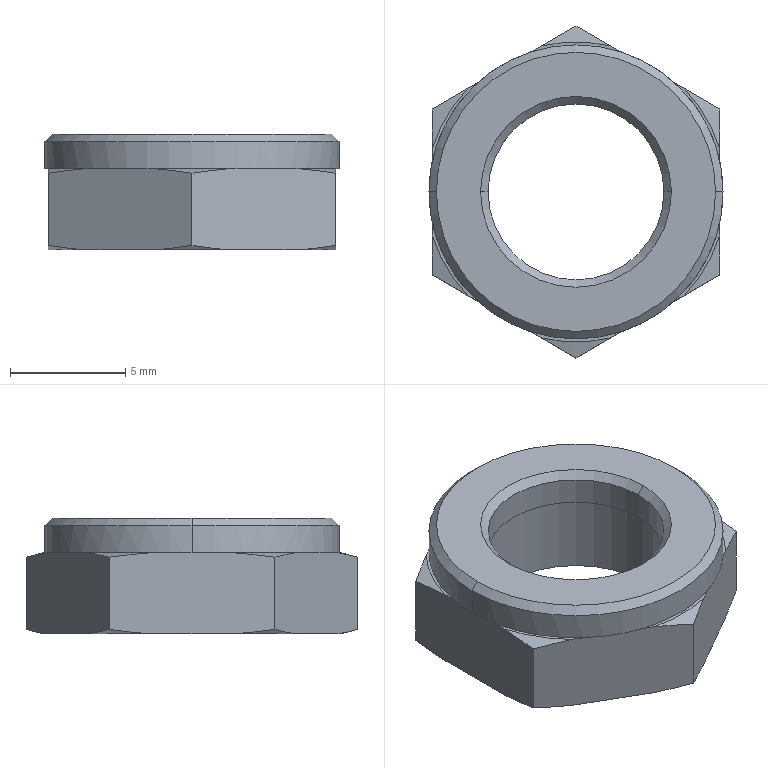Part | SolidWorks | features Cut 3, Boss 1, Chamfer 1, Extrusion 1 | 1 solid | 43 faces | box 12.74 x 14.38 x 5 mm | volume 412.934 mm3 | plane 21 | cone 16 | cylinder 6 | commonest cylinder face diameters 7.619 x2 8 x2 12.74 x2
STEP:
#1=CARTESIAN_POINT('',(-3.81,0.,4.675));
#2=VERTEX_POINT('',#1);
#3=CARTESIAN_POINT('',(3.81,0.,4.675));
#4=VERTEX_POINT('',#3);
#5=CARTESIAN_POINT('',(0.,0.,4.675));
#6=DIRECTION('',(0.,0.,1.));
#7=DIRECTION('',(1.,0.,0.));
#8=AXIS2_PLACEMENT_3D('',#5,#6,#7);
#9=CIRCLE('',#8,3.81);
#10=EDGE_CURVE('',#2,#4,#9,.T.);
#11=ORIENTED_EDGE('',*,*,#10,.F.);
#12=CARTESIAN_POINT('',(-4.135,0.,5.));
#13=VERTEX_POINT('',#12);
#14=CARTESIAN_POINT('',(-3.81,0.,4.675));
#15=DIRECTION('',(-0.7071,0.,0.7071));
#16=VECTOR('',#15,1000.);
#17=LINE('',#14,#16);
#18=EDGE_CURVE('',#2,#13,#17,.T.);
#19=ORIENTED_EDGE('',*,*,#18,.T.);
#20=CARTESIAN_POINT('',(4.135,0.,5.));
#21=VERTEX_POINT('',#20);
#22=CARTESIAN_POINT('',(0.,0.,5.));
#23=DIRECTION('',(0.,0.,-1.));
#24=DIRECTION('',(1.,0.,0.));
#25=AXIS2_PLACEMENT_3D('',#22,#23,#24);
#26=CIRCLE('',#25,4.135);
#27=EDGE_CURVE('',#21,#13,#26,.T.);
#28=ORIENTED_EDGE('',*,*,#27,.F.);
#29=CARTESIAN_POINT('',(3.81,0.,4.675));
#30=DIRECTION('',(0.7071,0.,0.7071));
#31=VECTOR('',#30,1000.);
#32=LINE('',#29,#31);
#33=EDGE_CURVE('',#4,#21,#32,.T.);
#34=ORIENTED_EDGE('',*,*,#33,.F.);
#35=EDGE_LOOP('',(#11,#19,#28,#34));
#36=FACE_OUTER_BOUND('',#35,.T.);
#37=CARTESIAN_POINT('',(0.,0.,4.675));
#38=DIRECTION('',(0.,0.,1.));
#39=DIRECTION('',(1.,0.,0.));
#40=AXIS2_PLACEMENT_3D('',#37,#38,#39);
#41=CONICAL_SURFACE('',#40,3.81,0.7854);
#42=ADVANCED_FACE('',(#36),#41,.F.);
#43=CARTESIAN_POINT('',(6.045,0.,5.));
#44=VERTEX_POINT('',#43);
#45=CARTESIAN_POINT('',(-6.045,0.,5.));
#46=VERTEX_POINT('',#45);
#47=CARTESIAN_POINT('',(0.,0.,5.));
#48=DIRECTION('',(0.,0.,1.));
#49=DIRECTION('',(1.,0.,0.));
#50=AXIS2_PLACEMENT_3D('',#47,#48,#49);
#51=CIRCLE('',#50,6.045);
#52=EDGE_CURVE('',#44,#46,#51,.T.);
#53=ORIENTED_EDGE('',*,*,#52,.F.);
#54=CARTESIAN_POINT('',(6.37,0.,4.675));
#55=VERTEX_POINT('',#54);
#56=CARTESIAN_POINT('',(6.045,0.,5.));
#57=DIRECTION('',(0.7071,0.,-0.7071));
#58=VECTOR('',#57,1000.);
#59=LINE('',#56,#58);
#60=EDGE_CURVE('',#44,#55,#59,.T.);
#61=ORIENTED_EDGE('',*,*,#60,.T.);
#62=CARTESIAN_POINT('',(-6.37,0.,4.675));
#63=VERTEX_POINT('',#62);
#64=CARTESIAN_POINT('',(0.,0.,4.675));
#65=DIRECTION('',(0.,0.,-1.));
#66=DIRECTION('',(1.,0.,0.));
#67=AXIS2_PLACEMENT_3D('',#64,#65,#66);
#68=CIRCLE('',#67,6.37);
#69=EDGE_CURVE('',#63,#55,#68,.T.);
#70=ORIENTED_EDGE('',*,*,#69,.F.);
#71=CARTESIAN_POINT('',(-6.045,0.,5.));
#72=DIRECTION('',(-0.7071,0.,-0.7071));
#73=VECTOR('',#72,1000.);
#74=LINE('',#71,#73);
#75=EDGE_CURVE('',#46,#63,#74,.T.);
#76=ORIENTED_EDGE('',*,*,#75,.F.);
#77=EDGE_LOOP('',(#53,#61,#70,#76));
#78=FACE_OUTER_BOUND('',#77,.T.);
#79=CARTESIAN_POINT('',(0.,0.,5.));
#80=DIRECTION('',(0.,0.,-1.));
#81=DIRECTION('',(-1.,0.,0.));
#82=AXIS2_PLACEMENT_3D('',#79,#80,#81);
#83=CONICAL_SURFACE('',#82,6.045,0.7854);
#84=ADVANCED_FACE('',(#78),#83,.T.);
#85=CARTESIAN_POINT('',(-3.81,0.,3.5));
#86=VERTEX_POINT('',#85);
#87=CARTESIAN_POINT('',(3.81,0.,3.5));
#88=VERTEX_POINT('',#87);
#89=CARTESIAN_POINT('',(0.,0.,3.5));
#90=DIRECTION('',(0.,0.,1.));
#91=DIRECTION('',(1.,0.,0.));
#92=AXIS2_PLACEMENT_3D('',#89,#90,#91);
#93=CIRCLE('',#92,3.81);
#94=EDGE_CURVE('',#86,#88,#93,.T.);
#95=ORIENTED_EDGE('',*,*,#94,.F.);
#96=CARTESIAN_POINT('',(-3.81,0.,0.));
#97=DIRECTION('',(0.,0.,1.));
#98=VECTOR('',#97,1000.);
#99=LINE('',#96,#98);
#100=EDGE_CURVE('',#86,#2,#99,.T.);
#101=ORIENTED_EDGE('',*,*,#100,.T.);
#102=ORIENTED_EDGE('',*,*,#10,.T.);
#103=CARTESIAN_POINT('',(3.81,0.,0.));
#104=DIRECTION('',(0.,0.,1.));
#105=VECTOR('',#104,1000.);
#106=LINE('',#103,#105);
#107=EDGE_CURVE('',#88,#4,#106,.T.);
#108=ORIENTED_EDGE('',*,*,#107,.F.);
#109=EDGE_LOOP('',(#95,#101,#102,#108));
#110=FACE_OUTER_BOUND('',#109,.T.);
#111=CARTESIAN_POINT('',(0.,0.,0.));
#112=DIRECTION('',(0.,0.,1.));
#113=DIRECTION('',(1.,0.,0.));
#114=AXIS2_PLACEMENT_3D('',#111,#112,#113);
#115=CYLINDRICAL_SURFACE('',#114,3.81);
#116=ADVANCED_FACE('',(#110),#115,.F.);
#117=ORIENTED_EDGE('',*,*,#69,.T.);
#118=CARTESIAN_POINT('',(6.37,0.,3.5));
#119=VERTEX_POINT('',#118);
#120=CARTESIAN_POINT('',(6.37,0.,5.));
#121=DIRECTION('',(0.,0.,-1.));
#122=VECTOR('',#121,1000.);
#123=LINE('',#120,#122);
#124=EDGE_CURVE('',#55,#119,#123,.T.);
#125=ORIENTED_EDGE('',*,*,#124,.T.);
#126=CARTESIAN_POINT('',(6.227,1.343,3.5));
#127=VERTEX_POINT('',#126);
#128=CARTESIAN_POINT('',(0.,0.,3.5));
#129=DIRECTION('',(0.,0.,1.));
#130=DIRECTION('',(1.,0.,0.));
#131=AXIS2_PLACEMENT_3D('',#128,#129,#130);
#132=CIRCLE('',#131,6.37);
#133=EDGE_CURVE('',#119,#127,#132,.T.);
#134=ORIENTED_EDGE('',*,*,#133,.T.);
#135=CARTESIAN_POINT('',(4.277,4.721,3.5));
#136=VERTEX_POINT('',#135);
#137=CARTESIAN_POINT('',(0.,0.,3.5));
#138=DIRECTION('',(0.,0.,1.));
#139=DIRECTION('',(1.,0.,0.));
#140=AXIS2_PLACEMENT_3D('',#137,#138,#139);
#141=CIRCLE('',#140,6.37);
#142=EDGE_CURVE('',#127,#136,#141,.T.);
#143=ORIENTED_EDGE('',*,*,#142,.T.);
#144=CARTESIAN_POINT('',(1.95,6.064,3.5));
#145=VERTEX_POINT('',#144);
#146=CARTESIAN_POINT('',(0.,0.,3.5));
#147=DIRECTION('',(0.,0.,1.));
#148=DIRECTION('',(1.,0.,0.));
#149=AXIS2_PLACEMENT_3D('',#146,#147,#148);
#150=CIRCLE('',#149,6.37);
#151=EDGE_CURVE('',#136,#145,#150,.T.);
#152=ORIENTED_EDGE('',*,*,#151,.T.);
#153=CARTESIAN_POINT('',(-1.95,6.064,3.5));
#154=VERTEX_POINT('',#153);
#155=CARTESIAN_POINT('',(0.,0.,3.5));
#156=DIRECTION('',(0.,0.,1.));
#157=DIRECTION('',(1.,0.,0.));
#158=AXIS2_PLACEMENT_3D('',#155,#156,#157);
#159=CIRCLE('',#158,6.37);
#160=EDGE_CURVE('',#145,#154,#159,.T.);
#161=ORIENTED_EDGE('',*,*,#160,.T.);
#162=CARTESIAN_POINT('',(-4.277,4.721,3.5));
#163=VERTEX_POINT('',#162);
#164=CARTESIAN_POINT('',(0.,0.,3.5));
#165=DIRECTION('',(0.,0.,1.));
#166=DIRECTION('',(1.,0.,0.));
#167=AXIS2_PLACEMENT_3D('',#164,#165,#166);
#168=CIRCLE('',#167,6.37);
#169=EDGE_CURVE('',#154,#163,#168,.T.);
#170=ORIENTED_EDGE('',*,*,#169,.T.);
#171=CARTESIAN_POINT('',(-6.227,1.343,3.5));
#172=VERTEX_POINT('',#171);
#173=CARTESIAN_POINT('',(0.,0.,3.5));
#174=DIRECTION('',(0.,0.,1.));
#175=DIRECTION('',(1.,0.,0.));
#176=AXIS2_PLACEMENT_3D('',#173,#174,#175);
#177=CIRCLE('',#176,6.37);
#178=EDGE_CURVE('',#163,#172,#177,.T.);
#179=ORIENTED_EDGE('',*,*,#178,.T.);
#180=CARTESIAN_POINT('',(-6.37,0.,3.5));
#181=VERTEX_POINT('',#180);
#182=CARTESIAN_POINT('',(0.,0.,3.5));
#183=DIRECTION('',(0.,0.,1.));
#184=DIRECTION('',(1.,0.,0.));
#185=AXIS2_PLACEMENT_3D('',#182,#183,#184);
#186=CIRCLE('',#185,6.37);
#187=EDGE_CURVE('',#172,#181,#186,.T.);
#188=ORIENTED_EDGE('',*,*,#187,.T.);
#189=CARTESIAN_POINT('',(-6.37,0.,5.));
#190=DIRECTION('',(0.,0.,-1.));
#191=VECTOR('',#190,1000.);
#192=LINE('',#189,#191);
#193=EDGE_CURVE('',#63,#181,#192,.T.);
#194=ORIENTED_EDGE('',*,*,#193,.F.);
#195=EDGE_LOOP('',(#117,#125,#134,#143,#152,#161,#170,#179,#188,#194));
#196=FACE_OUTER_BOUND('',#195,.T.);
#197=CARTESIAN_POINT('',(0.,0.,5.));
#198=DIRECTION('',(0.,0.,-1.));
#199=DIRECTION('',(-1.,0.,0.));
#200=AXIS2_PLACEMENT_3D('',#197,#198,#199);
#201=CYLINDRICAL_SURFACE('',#200,6.37);
#202=ADVANCED_FACE('',(#196),#201,.T.);
#203=CARTESIAN_POINT('',(-4.,0.,3.5));
#204=VERTEX_POINT('',#203);
#205=CARTESIAN_POINT('',(4.,0.,3.5));
#206=VERTEX_POINT('',#205);
#207=CARTESIAN_POINT('',(0.,0.,3.5));
#208=DIRECTION('',(0.,0.,1.));
#209=DIRECTION('',(1.,0.,0.));
#210=AXIS2_PLACEMENT_3D('',#207,#208,#209);
#211=CIRCLE('',#210,4.);
#212=EDGE_CURVE('',#204,#206,#211,.T.);
#213=ORIENTED_EDGE('',*,*,#212,.T.);
#214=CARTESIAN_POINT('',(4.,0.,0.));
#215=VERTEX_POINT('',#214);
#216=CARTESIAN_POINT('',(4.,0.,3.5));
#217=DIRECTION('',(0.,0.,-1.));
#218=VECTOR('',#217,1000.);
#219=LINE('',#216,#218);
#220=EDGE_CURVE('',#206,#215,#219,.T.);
#221=ORIENTED_EDGE('',*,*,#220,.T.);
#222=CARTESIAN_POINT('',(-4.,0.,0.));
#223=VERTEX_POINT('',#222);
#224=CARTESIAN_POINT('',(0.,0.,0.));
#225=DIRECTION('',(0.,0.,1.));
#226=DIRECTION('',(1.,0.,0.));
#227=AXIS2_PLACEMENT_3D('',#224,#225,#226);
#228=CIRCLE('',#227,4.);
#229=EDGE_CURVE('',#223,#215,#228,.T.);
#230=ORIENTED_EDGE('',*,*,#229,.F.);
#231=CARTESIAN_POINT('',(-4.,0.,3.5));
#232=DIRECTION('',(0.,0.,-1.));
#233=VECTOR('',#232,1000.);
#234=LINE('',#231,#233);
#235=EDGE_CURVE('',#204,#223,#234,.T.);
#236=ORIENTED_EDGE('',*,*,#235,.F.);
#237=EDGE_LOOP('',(#213,#221,#230,#236));
#238=FACE_OUTER_BOUND('',#237,.T.);
#239=CARTESIAN_POINT('',(0.,0.,3.5));
#240=DIRECTION('',(0.,0.,-1.));
#241=DIRECTION('',(-1.,0.,0.));
#242=AXIS2_PLACEMENT_3D('',#239,#240,#241);
#243=CYLINDRICAL_SURFACE('',#242,4.);
#244=ADVANCED_FACE('',(#238),#243,.F.);
#245=CARTESIAN_POINT('',(-6.227,-1.343,3.5));
#246=VERTEX_POINT('',#245);
#247=CARTESIAN_POINT('',(-4.277,-4.721,3.5));
#248=VERTEX_POINT('',#247);
#249=CARTESIAN_POINT('',(0.,0.,3.5));
#250=DIRECTION('',(0.,0.,1.));
#251=DIRECTION('',(1.,0.,0.));
#252=AXIS2_PLACEMENT_3D('',#249,#250,#251);
#253=CIRCLE('',#252,6.37);
#254=EDGE_CURVE('',#246,#248,#253,.T.);
#255=ORIENTED_EDGE('',*,*,#254,.F.);
#256=CARTESIAN_POINT('',(-6.227,-1.865,3.5));
#257=VERTEX_POINT('',#256);
#258=CARTESIAN_POINT('',(-6.227,3.595,3.5));
#259=DIRECTION('',(0.,-1.,0.));
#260=VECTOR('',#259,1000.);
#261=LINE('',#258,#260);
#262=EDGE_CURVE('',#246,#257,#261,.T.);
#263=ORIENTED_EDGE('',*,*,#262,.T.);
#264=CARTESIAN_POINT('',(-4.728,-4.46,3.5));
#265=VERTEX_POINT('',#264);
#266=CARTESIAN_POINT('',(0.,0.,3.5));
#267=DIRECTION('',(0.,0.,1.));
#268=DIRECTION('',(1.,0.,0.));
#269=AXIS2_PLACEMENT_3D('',#266,#267,#268);
#270=CIRCLE('',#269,6.5);
#271=EDGE_CURVE('',#257,#265,#270,.T.);
#272=ORIENTED_EDGE('',*,*,#271,.T.);
#273=CARTESIAN_POINT('',(-6.227,-3.595,3.5));
#274=DIRECTION('',(0.866,-0.5,0.));
#275=VECTOR('',#274,1000.);
#276=LINE('',#273,#275);
#277=EDGE_CURVE('',#265,#248,#276,.T.);
#278=ORIENTED_EDGE('',*,*,#277,.T.);
#279=EDGE_LOOP('',(#255,#263,#272,#278));
#280=FACE_OUTER_BOUND('',#279,.T.);
#281=CARTESIAN_POINT('',(6.227,3.595,3.5));
#282=DIRECTION('',(0.,0.,-1.));
#283=DIRECTION('',(-1.,0.,0.));
#284=AXIS2_PLACEMENT_3D('',#281,#282,#283);
#285=PLANE('',#284);
#286=ADVANCED_FACE('',(#280),#285,.F.);
#287=CARTESIAN_POINT('',(-1.95,-6.064,3.5));
#288=VERTEX_POINT('',#287);
#289=CARTESIAN_POINT('',(1.95,-6.064,3.5));
#290=VERTEX_POINT('',#289);
#291=CARTESIAN_POINT('',(0.,0.,3.5));
#292=DIRECTION('',(0.,0.,1.));
#293=DIRECTION('',(1.,0.,0.));
#294=AXIS2_PLACEMENT_3D('',#291,#292,#293);
#295=CIRCLE('',#294,6.37);
#296=EDGE_CURVE('',#288,#290,#295,.T.);
#297=ORIENTED_EDGE('',*,*,#296,.F.);
#298=CARTESIAN_POINT('',(-1.498,-6.325,3.5));
#299=VERTEX_POINT('',#298);
#300=CARTESIAN_POINT('',(-6.227,-3.595,3.5));
#301=DIRECTION('',(0.866,-0.5,0.));
#302=VECTOR('',#301,1000.);
#303=LINE('',#300,#302);
#304=EDGE_CURVE('',#288,#299,#303,.T.);
#305=ORIENTED_EDGE('',*,*,#304,.T.);
#306=CARTESIAN_POINT('',(1.498,-6.325,3.5));
#307=VERTEX_POINT('',#306);
#308=CARTESIAN_POINT('',(0.,0.,3.5));
#309=DIRECTION('',(0.,0.,1.));
#310=DIRECTION('',(1.,0.,0.));
#311=AXIS2_PLACEMENT_3D('',#308,#309,#310);
#312=CIRCLE('',#311,6.5);
#313=EDGE_CURVE('',#299,#307,#312,.T.);
#314=ORIENTED_EDGE('',*,*,#313,.T.);
#315=CARTESIAN_POINT('',(0.,-7.19,3.5));
#316=DIRECTION('',(0.866,0.5,0.));
#317=VECTOR('',#316,1000.);
#318=LINE('',#315,#317);
#319=EDGE_CURVE('',#307,#290,#318,.T.);
#320=ORIENTED_EDGE('',*,*,#319,.T.);
#321=EDGE_LOOP('',(#297,#305,#314,#320));
#322=FACE_OUTER_BOUND('',#321,.T.);
#323=CARTESIAN_POINT('',(6.227,3.595,3.5));
#324=DIRECTION('',(0.,0.,-1.));
#325=DIRECTION('',(-1.,0.,0.));
#326=AXIS2_PLACEMENT_3D('',#323,#324,#325);
#327=PLANE('',#326);
#328=ADVANCED_FACE('',(#322),#327,.F.);
#329=CARTESIAN_POINT('',(4.277,-4.721,3.5));
#330=VERTEX_POINT('',#329);
#331=CARTESIAN_POINT('',(6.227,-1.343,3.5));
#332=VERTEX_POINT('',#331);
#333=CARTESIAN_POINT('',(0.,0.,3.5));
#334=DIRECTION('',(0.,0.,1.));
#335=DIRECTION('',(1.,0.,0.));
#336=AXIS2_PLACEMENT_3D('',#333,#334,#335);
#337=CIRCLE('',#336,6.37);
#338=EDGE_CURVE('',#330,#332,#337,.T.);
#339=ORIENTED_EDGE('',*,*,#338,.F.);
#340=CARTESIAN_POINT('',(4.728,-4.46,3.5));
#341=VERTEX_POINT('',#340);
#342=CARTESIAN_POINT('',(0.,-7.19,3.5));
#343=DIRECTION('',(0.866,0.5,0.));
#344=VECTOR('',#343,1000.);
#345=LINE('',#342,#344);
#346=EDGE_CURVE('',#330,#341,#345,.T.);
#347=ORIENTED_EDGE('',*,*,#346,.T.);
#348=CARTESIAN_POINT('',(6.227,-1.865,3.5));
#349=VERTEX_POINT('',#348);
#350=CARTESIAN_POINT('',(0.,0.,3.5));
#351=DIRECTION('',(0.,0.,1.));
#352=DIRECTION('',(1.,0.,0.));
#353=AXIS2_PLACEMENT_3D('',#350,#351,#352);
#354=CIRCLE('',#353,6.5);
#355=EDGE_CURVE('',#341,#349,#354,.T.);
#356=ORIENTED_EDGE('',*,*,#355,.T.);
#357=CARTESIAN_POINT('',(6.227,-3.595,3.5));
#358=DIRECTION('',(0.,1.,0.));
#359=VECTOR('',#358,1000.);
#360=LINE('',#357,#359);
#361=EDGE_CURVE('',#349,#332,#360,.T.);
#362=ORIENTED_EDGE('',*,*,#361,.T.);
#363=EDGE_LOOP('',(#339,#347,#356,#362));
#364=FACE_OUTER_BOUND('',#363,.T.);
#365=CARTESIAN_POINT('',(6.227,3.595,3.5));
#366=DIRECTION('',(0.,0.,-1.));
#367=DIRECTION('',(-1.,0.,0.));
#368=AXIS2_PLACEMENT_3D('',#365,#366,#367);
#369=PLANE('',#368);
#370=ADVANCED_FACE('',(#364),#369,.F.);
#371=ORIENTED_EDGE('',*,*,#142,.F.);
#372=CARTESIAN_POINT('',(6.227,1.865,3.5));
#373=VERTEX_POINT('',#372);
#374=CARTESIAN_POINT('',(6.227,-3.595,3.5));
#375=DIRECTION('',(0.,1.,0.));
#376=VECTOR('',#375,1000.);
#377=LINE('',#374,#376);
#378=EDGE_CURVE('',#127,#373,#377,.T.);
#379=ORIENTED_EDGE('',*,*,#378,.T.);
#380=CARTESIAN_POINT('',(4.728,4.46,3.5));
#381=VERTEX_POINT('',#380);
#382=CARTESIAN_POINT('',(0.,0.,3.5));
#383=DIRECTION('',(0.,0.,1.));
#384=DIRECTION('',(1.,0.,0.));
#385=AXIS2_PLACEMENT_3D('',#382,#383,#384);
#386=CIRCLE('',#385,6.5);
#387=EDGE_CURVE('',#373,#381,#386,.T.);
#388=ORIENTED_EDGE('',*,*,#387,.T.);
#389=CARTESIAN_POINT('',(6.227,3.595,3.5));
#390=DIRECTION('',(-0.866,0.5,0.));
#391=VECTOR('',#390,1000.);
#392=LINE('',#389,#391);
#393=EDGE_CURVE('',#381,#136,#392,.T.);
#394=ORIENTED_EDGE('',*,*,#393,.T.);
#395=EDGE_LOOP('',(#371,#379,#388,#394));
#396=FACE_OUTER_BOUND('',#395,.T.);
#397=CARTESIAN_POINT('',(6.227,3.595,3.5));
#398=DIRECTION('',(0.,0.,-1.));
#399=DIRECTION('',(-1.,0.,0.));
#400=AXIS2_PLACEMENT_3D('',#397,#398,#399);
#401=PLANE('',#400);
#402=ADVANCED_FACE('',(#396),#401,.F.);
#403=ORIENTED_EDGE('',*,*,#160,.F.);
#404=CARTESIAN_POINT('',(1.498,6.325,3.5));
#405=VERTEX_POINT('',#404);
#406=CARTESIAN_POINT('',(6.227,3.595,3.5));
#407=DIRECTION('',(-0.866,0.5,0.));
#408=VECTOR('',#407,1000.);
#409=LINE('',#406,#408);
#410=EDGE_CURVE('',#145,#405,#409,.T.);
#411=ORIENTED_EDGE('',*,*,#410,.T.);
#412=CARTESIAN_POINT('',(-1.498,6.325,3.5));
#413=VERTEX_POINT('',#412);
#414=CARTESIAN_POINT('',(0.,0.,3.5));
#415=DIRECTION('',(0.,0.,1.));
#416=DIRECTION('',(1.,0.,0.));
#417=AXIS2_PLACEMENT_3D('',#414,#415,#416);
#418=CIRCLE('',#417,6.5);
#419=EDGE_CURVE('',#405,#413,#418,.T.);
#420=ORIENTED_EDGE('',*,*,#419,.T.);
#421=CARTESIAN_POINT('',(0.,7.19,3.5));
#422=DIRECTION('',(-0.866,-0.5,0.));
#423=VECTOR('',#422,1000.);
#424=LINE('',#421,#423);
#425=EDGE_CURVE('',#413,#154,#424,.T.);
#426=ORIENTED_EDGE('',*,*,#425,.T.);
#427=EDGE_LOOP('',(#403,#411,#420,#426));
#428=FACE_OUTER_BOUND('',#427,.T.);
#429=CARTESIAN_POINT('',(6.227,3.595,3.5));
#430=DIRECTION('',(0.,0.,-1.));
#431=DIRECTION('',(-1.,0.,0.));
#432=AXIS2_PLACEMENT_3D('',#429,#430,#431);
#433=PLANE('',#432);
#434=ADVANCED_FACE('',(#428),#433,.F.);
#435=ORIENTED_EDGE('',*,*,#178,.F.);
#436=CARTESIAN_POINT('',(-4.728,4.46,3.5));
#437=VERTEX_POINT('',#436);
#438=CARTESIAN_POINT('',(0.,7.19,3.5));
#439=DIRECTION('',(-0.866,-0.5,0.));
#440=VECTOR('',#439,1000.);
#441=LINE('',#438,#440);
#442=EDGE_CURVE('',#163,#437,#441,.T.);
#443=ORIENTED_EDGE('',*,*,#442,.T.);
#444=CARTESIAN_POINT('',(-6.227,1.865,3.5));
#445=VERTEX_POINT('',#444);
#446=CARTESIAN_POINT('',(0.,0.,3.5));
#447=DIRECTION('',(0.,0.,1.));
#448=DIRECTION('',(1.,0.,0.));
#449=AXIS2_PLACEMENT_3D('',#446,#447,#448);
#450=CIRCLE('',#449,6.5);
#451=EDGE_CURVE('',#437,#445,#450,.T.);
#452=ORIENTED_EDGE('',*,*,#451,.T.);
#453=CARTESIAN_POINT('',(-6.227,3.595,3.5));
#454=DIRECTION('',(0.,-1.,0.));
#455=VECTOR('',#454,1000.);
#456=LINE('',#453,#455);
#457=EDGE_CURVE('',#445,#172,#456,.T.);
#458=ORIENTED_EDGE('',*,*,#457,.T.);
#459=EDGE_LOOP('',(#435,#443,#452,#458));
#460=FACE_OUTER_BOUND('',#459,.T.);
#461=CARTESIAN_POINT('',(6.227,3.595,3.5));
#462=DIRECTION('',(0.,0.,-1.));
#463=DIRECTION('',(-1.,0.,0.));
#464=AXIS2_PLACEMENT_3D('',#461,#462,#463);
#465=PLANE('',#464);
#466=ADVANCED_FACE('',(#460),#465,.F.);
#467=CARTESIAN_POINT('',(0.,7.19,0.1849));
#468=VERTEX_POINT('',#467);
#469=CARTESIAN_POINT('',(1.498,6.325,0.));
#470=VERTEX_POINT('',#469);
#471=CARTESIAN_POINT('',(0.,7.19,0.1849));
#472=CARTESIAN_POINT('',(0.498,6.902,0.1078));
#473=CARTESIAN_POINT('',(0.9973,6.614,0.04448));
#474=CARTESIAN_POINT('',(1.498,6.325,0.));
#475=B_SPLINE_CURVE_WITH_KNOTS('',3,(#471,#472,#473,#474),.UNSPECIFIED.,.F.,.F.,(4,4),(0.005619,0.007359),.UNSPECIFIED.);
#476=EDGE_CURVE('',#468,#470,#475,.T.);
#477=ORIENTED_EDGE('',*,*,#476,.F.);
#478=CARTESIAN_POINT('',(0.,7.19,3.315));
#479=VERTEX_POINT('',#478);
#480=CARTESIAN_POINT('',(0.,7.19,3.5));
#481=DIRECTION('',(0.,0.,-1.));
#482=VECTOR('',#481,1000.);
#483=LINE('',#480,#482);
#484=EDGE_CURVE('',#479,#468,#483,.T.);
#485=ORIENTED_EDGE('',*,*,#484,.F.);
#486=CARTESIAN_POINT('',(1.498,6.325,3.5));
#487=CARTESIAN_POINT('',(0.9975,6.614,3.456));
#488=CARTESIAN_POINT('',(0.4973,6.903,3.392));
#489=CARTESIAN_POINT('',(0.,7.19,3.315));
#490=B_SPLINE_CURVE_WITH_KNOTS('',3,(#486,#487,#488,#489),.UNSPECIFIED.,.F.,.F.,(4,4),(0.01107,0.01278),.UNSPECIFIED.);
#491=EDGE_CURVE('',#405,#479,#490,.T.);
#492=ORIENTED_EDGE('',*,*,#491,.F.);
#493=ORIENTED_EDGE('',*,*,#410,.F.);
#494=CARTESIAN_POINT('',(6.227,3.595,3.5));
#495=DIRECTION('',(-0.866,0.5,0.));
#496=VECTOR('',#495,1000.);
#497=LINE('',#494,#496);
#498=EDGE_CURVE('',#136,#145,#497,.T.);
#499=ORIENTED_EDGE('',*,*,#498,.F.);
#500=ORIENTED_EDGE('',*,*,#393,.F.);
#501=CARTESIAN_POINT('',(6.227,3.595,3.315));
#502=VERTEX_POINT('',#501);
#503=CARTESIAN_POINT('',(6.227,3.595,3.315));
#504=CARTESIAN_POINT('',(5.729,3.883,3.392));
#505=CARTESIAN_POINT('',(5.229,4.171,3.456));
#506=CARTESIAN_POINT('',(4.728,4.46,3.5));
#507=B_SPLINE_CURVE_WITH_KNOTS('',3,(#503,#504,#505,#506),.UNSPECIFIED.,.F.,.F.,(4,4),(0.005619,0.007359),.UNSPECIFIED.);
#508=EDGE_CURVE('',#502,#381,#507,.T.);
#509=ORIENTED_EDGE('',*,*,#508,.F.);
#510=CARTESIAN_POINT('',(6.227,3.595,0.1849));
#511=VERTEX_POINT('',#510);
#512=CARTESIAN_POINT('',(6.227,3.595,3.5));
#513=DIRECTION('',(0.,0.,-1.));
#514=VECTOR('',#513,1000.);
#515=LINE('',#512,#514);
#516=EDGE_CURVE('',#502,#511,#515,.T.);
#517=ORIENTED_EDGE('',*,*,#516,.T.);
#518=CARTESIAN_POINT('',(4.728,4.46,0.));
#519=VERTEX_POINT('',#518);
#520=CARTESIAN_POINT('',(4.728,4.46,0.));
#521=CARTESIAN_POINT('',(5.229,4.171,0.04445));
#522=CARTESIAN_POINT('',(5.729,3.882,0.108));
#523=CARTESIAN_POINT('',(6.227,3.595,0.1849));
#524=B_SPLINE_CURVE_WITH_KNOTS('',3,(#520,#521,#522,#523),.UNSPECIFIED.,.F.,.F.,(4,4),(0.01107,0.01278),.UNSPECIFIED.);
#525=EDGE_CURVE('',#519,#511,#524,.T.);
#526=ORIENTED_EDGE('',*,*,#525,.F.);
#527=CARTESIAN_POINT('',(6.227,3.595,0.));
#528=DIRECTION('',(-0.866,0.5,0.));
#529=VECTOR('',#528,1000.);
#530=LINE('',#527,#529);
#531=EDGE_CURVE('',#519,#470,#530,.T.);
#532=ORIENTED_EDGE('',*,*,#531,.T.);
#533=EDGE_LOOP('',(#477,#485,#492,#493,#499,#500,#509,#517,#526,#532));
#534=FACE_OUTER_BOUND('',#533,.T.);
#535=CARTESIAN_POINT('',(6.227,3.595,3.5));
#536=DIRECTION('',(-0.5,-0.866,0.));
#537=DIRECTION('',(0.866,-0.5,0.));
#538=AXIS2_PLACEMENT_3D('',#535,#536,#537);
#539=PLANE('',#538);
#540=ADVANCED_FACE('',(#534),#539,.F.);
#541=CARTESIAN_POINT('',(-6.227,3.595,0.1849));
#542=VERTEX_POINT('',#541);
#543=CARTESIAN_POINT('',(-4.728,4.46,0.));
#544=VERTEX_POINT('',#543);
#545=CARTESIAN_POINT('',(-6.227,3.595,0.1849));
#546=CARTESIAN_POINT('',(-5.729,3.883,0.1078));
#547=CARTESIAN_POINT('',(-5.229,4.171,0.04448));
#548=CARTESIAN_POINT('',(-4.728,4.46,0.));
#549=B_SPLINE_CURVE_WITH_KNOTS('',3,(#545,#546,#547,#548),.UNSPECIFIED.,.F.,.F.,(4,4),(0.005619,0.007359),.UNSPECIFIED.);
#550=EDGE_CURVE('',#542,#544,#549,.T.);
#551=ORIENTED_EDGE('',*,*,#550,.F.);
#552=CARTESIAN_POINT('',(-6.227,3.595,3.315));
#553=VERTEX_POINT('',#552);
#554=CARTESIAN_POINT('',(-6.227,3.595,3.5));
#555=DIRECTION('',(0.,0.,-1.));
#556=VECTOR('',#555,1000.);
#557=LINE('',#554,#556);
#558=EDGE_CURVE('',#553,#542,#557,.T.);
#559=ORIENTED_EDGE('',*,*,#558,.F.);
#560=CARTESIAN_POINT('',(-4.728,4.46,3.5));
#561=CARTESIAN_POINT('',(-5.229,4.171,3.456));
#562=CARTESIAN_POINT('',(-5.729,3.882,3.392));
#563=CARTESIAN_POINT('',(-6.227,3.595,3.315));
#564=B_SPLINE_CURVE_WITH_KNOTS('',3,(#560,#561,#562,#563),.UNSPECIFIED.,.F.,.F.,(4,4),(0.01107,0.01278),.UNSPECIFIED.);
#565=EDGE_CURVE('',#437,#553,#564,.T.);
#566=ORIENTED_EDGE('',*,*,#565,.F.);
#567=ORIENTED_EDGE('',*,*,#442,.F.);
#568=CARTESIAN_POINT('',(0.,7.19,3.5));
#569=DIRECTION('',(-0.866,-0.5,0.));
#570=VECTOR('',#569,1000.);
#571=LINE('',#568,#570);
#572=EDGE_CURVE('',#154,#163,#571,.T.);
#573=ORIENTED_EDGE('',*,*,#572,.F.);
#574=ORIENTED_EDGE('',*,*,#425,.F.);
#575=CARTESIAN_POINT('',(0.,7.19,3.315));
#576=CARTESIAN_POINT('',(-0.498,6.902,3.392));
#577=CARTESIAN_POINT('',(-0.9973,6.614,3.456));
#578=CARTESIAN_POINT('',(-1.498,6.325,3.5));
#579=B_SPLINE_CURVE_WITH_KNOTS('',3,(#575,#576,#577,#578),.UNSPECIFIED.,.F.,.F.,(4,4),(0.005619,0.007359),.UNSPECIFIED.);
#580=EDGE_CURVE('',#479,#413,#579,.T.);
#581=ORIENTED_EDGE('',*,*,#580,.F.);
#582=ORIENTED_EDGE('',*,*,#484,.T.);
#583=CARTESIAN_POINT('',(-1.498,6.325,0.));
#584=VERTEX_POINT('',#583);
#585=CARTESIAN_POINT('',(-1.498,6.325,0.));
#586=CARTESIAN_POINT('',(-0.9975,6.614,0.04445));
#587=CARTESIAN_POINT('',(-0.4973,6.903,0.108));
#588=CARTESIAN_POINT('',(0.,7.19,0.1849));
#589=B_SPLINE_CURVE_WITH_KNOTS('',3,(#585,#586,#587,#588),.UNSPECIFIED.,.F.,.F.,(4,4),(0.01107,0.01278),.UNSPECIFIED.);
#590=EDGE_CURVE('',#584,#468,#589,.T.);
#591=ORIENTED_EDGE('',*,*,#590,.F.);
#592=CARTESIAN_POINT('',(0.,7.19,0.));
#593=DIRECTION('',(-0.866,-0.5,0.));
#594=VECTOR('',#593,1000.);
#595=LINE('',#592,#594);
#596=EDGE_CURVE('',#584,#544,#595,.T.);
#597=ORIENTED_EDGE('',*,*,#596,.T.);
#598=EDGE_LOOP('',(#551,#559,#566,#567,#573,#574,#581,#582,#591,#597));
#599=FACE_OUTER_BOUND('',#598,.T.);
#600=CARTESIAN_POINT('',(0.,7.19,3.5));
#601=DIRECTION('',(0.5,-0.866,0.));
#602=DIRECTION('',(0.866,0.5,0.));
#603=AXIS2_PLACEMENT_3D('',#600,#601,#602);
#604=PLANE('',#603);
#605=ADVANCED_FACE('',(#599),#604,.F.);
#606=CARTESIAN_POINT('',(-6.227,-3.595,0.1849));
#607=VERTEX_POINT('',#606);
#608=CARTESIAN_POINT('',(-6.227,-1.865,0.));
#609=VERTEX_POINT('',#608);
#610=CARTESIAN_POINT('',(-6.227,-3.595,0.1849));
#611=CARTESIAN_POINT('',(-6.227,-3.02,0.1078));
#612=CARTESIAN_POINT('',(-6.227,-2.443,0.04446));
#613=CARTESIAN_POINT('',(-6.227,-1.865,0.));
#614=B_SPLINE_CURVE_WITH_KNOTS('',3,(#610,#611,#612,#613),.UNSPECIFIED.,.F.,.F.,(4,4),(0.00486,0.0066),.UNSPECIFIED.);
#615=EDGE_CURVE('',#607,#609,#614,.T.);
#616=ORIENTED_EDGE('',*,*,#615,.F.);
#617=CARTESIAN_POINT('',(-6.227,-3.595,3.315));
#618=VERTEX_POINT('',#617);
#619=CARTESIAN_POINT('',(-6.227,-3.595,3.5));
#620=DIRECTION('',(0.,0.,-1.));
#621=VECTOR('',#620,1000.);
#622=LINE('',#619,#621);
#623=EDGE_CURVE('',#618,#607,#622,.T.);
#624=ORIENTED_EDGE('',*,*,#623,.F.);
#625=CARTESIAN_POINT('',(-6.227,-1.865,3.5));
#626=CARTESIAN_POINT('',(-6.227,-2.443,3.456));
#627=CARTESIAN_POINT('',(-6.227,-3.021,3.392));
#628=CARTESIAN_POINT('',(-6.227,-3.595,3.315));
#629=B_SPLINE_CURVE_WITH_KNOTS('',3,(#625,#626,#627,#628),.UNSPECIFIED.,.F.,.F.,(4,4),(0.01031,0.01202),.UNSPECIFIED.);
#630=EDGE_CURVE('',#257,#618,#629,.T.);
#631=ORIENTED_EDGE('',*,*,#630,.F.);
#632=ORIENTED_EDGE('',*,*,#262,.F.);
#633=CARTESIAN_POINT('',(-6.227,3.595,3.5));
#634=DIRECTION('',(0.,-1.,0.));
#635=VECTOR('',#634,1000.);
#636=LINE('',#633,#635);
#637=EDGE_CURVE('',#172,#246,#636,.T.);
#638=ORIENTED_EDGE('',*,*,#637,.F.);
#639=ORIENTED_EDGE('',*,*,#457,.F.);
#640=CARTESIAN_POINT('',(-6.227,3.595,3.315));
#641=CARTESIAN_POINT('',(-6.227,3.02,3.392));
#642=CARTESIAN_POINT('',(-6.227,2.443,3.456));
#643=CARTESIAN_POINT('',(-6.227,1.865,3.5));
#644=B_SPLINE_CURVE_WITH_KNOTS('',3,(#640,#641,#642,#643),.UNSPECIFIED.,.F.,.F.,(4,4),(0.00486,0.0066),.UNSPECIFIED.);
#645=EDGE_CURVE('',#553,#445,#644,.T.);
#646=ORIENTED_EDGE('',*,*,#645,.F.);
#647=ORIENTED_EDGE('',*,*,#558,.T.);
#648=CARTESIAN_POINT('',(-6.227,1.865,0.));
#649=VERTEX_POINT('',#648);
#650=CARTESIAN_POINT('',(-6.227,1.865,0.));
#651=CARTESIAN_POINT('',(-6.227,2.443,0.0444));
#652=CARTESIAN_POINT('',(-6.227,3.021,0.1079));
#653=CARTESIAN_POINT('',(-6.227,3.595,0.1849));
#654=B_SPLINE_CURVE_WITH_KNOTS('',3,(#650,#651,#652,#653),.UNSPECIFIED.,.F.,.F.,(4,4),(0.01031,0.01202),.UNSPECIFIED.);
#655=EDGE_CURVE('',#649,#542,#654,.T.);
#656=ORIENTED_EDGE('',*,*,#655,.F.);
#657=CARTESIAN_POINT('',(-6.227,3.595,0.));
#658=DIRECTION('',(0.,-1.,0.));
#659=VECTOR('',#658,1000.);
#660=LINE('',#657,#659);
#661=EDGE_CURVE('',#649,#609,#660,.T.);
#662=ORIENTED_EDGE('',*,*,#661,.T.);
#663=EDGE_LOOP('',(#616,#624,#631,#632,#638,#639,#646,#647,#656,#662));
#664=FACE_OUTER_BOUND('',#663,.T.);
#665=CARTESIAN_POINT('',(-6.227,3.595,3.5));
#666=DIRECTION('',(1.,0.,0.));
#667=DIRECTION('',(0.,0.,-1.));
#668=AXIS2_PLACEMENT_3D('',#665,#666,#667);
#669=PLANE('',#668);
#670=ADVANCED_FACE('',(#664),#669,.F.);
#671=CARTESIAN_POINT('',(0.,-7.19,0.1849));
#672=VERTEX_POINT('',#671);
#673=CARTESIAN_POINT('',(-1.498,-6.325,0.));
#674=VERTEX_POINT('',#673);
#675=CARTESIAN_POINT('',(0.,-7.19,0.1849));
#676=CARTESIAN_POINT('',(-0.498,-6.902,0.1078));
#677=CARTESIAN_POINT('',(-0.9973,-6.614,0.04448));
#678=CARTESIAN_POINT('',(-1.498,-6.325,0.));
#679=B_SPLINE_CURVE_WITH_KNOTS('',3,(#675,#676,#677,#678),.UNSPECIFIED.,.F.,.F.,(4,4),(0.005619,0.007359),.UNSPECIFIED.);
#680=EDGE_CURVE('',#672,#674,#679,.T.);
#681=ORIENTED_EDGE('',*,*,#680,.F.);
#682=CARTESIAN_POINT('',(0.,-7.19,3.315));
#683=VERTEX_POINT('',#682);
#684=CARTESIAN_POINT('',(0.,-7.19,3.5));
#685=DIRECTION('',(0.,0.,-1.));
#686=VECTOR('',#685,1000.);
#687=LINE('',#684,#686);
#688=EDGE_CURVE('',#683,#672,#687,.T.);
#689=ORIENTED_EDGE('',*,*,#688,.F.);
#690=CARTESIAN_POINT('',(-1.498,-6.325,3.5));
#691=CARTESIAN_POINT('',(-0.9975,-6.614,3.456));
#692=CARTESIAN_POINT('',(-0.4973,-6.903,3.392));
#693=CARTESIAN_POINT('',(0.,-7.19,3.315));
#694=B_SPLINE_CURVE_WITH_KNOTS('',3,(#690,#691,#692,#693),.UNSPECIFIED.,.F.,.F.,(4,4),(0.01107,0.01278),.UNSPECIFIED.);
#695=EDGE_CURVE('',#299,#683,#694,.T.);
#696=ORIENTED_EDGE('',*,*,#695,.F.);
#697=ORIENTED_EDGE('',*,*,#304,.F.);
#698=CARTESIAN_POINT('',(-6.227,-3.595,3.5));
#699=DIRECTION('',(0.866,-0.5,0.));
#700=VECTOR('',#699,1000.);
#701=LINE('',#698,#700);
#702=EDGE_CURVE('',#248,#288,#701,.T.);
#703=ORIENTED_EDGE('',*,*,#702,.F.);
#704=ORIENTED_EDGE('',*,*,#277,.F.);
#705=CARTESIAN_POINT('',(-6.227,-3.595,3.315));
#706=CARTESIAN_POINT('',(-5.729,-3.883,3.392));
#707=CARTESIAN_POINT('',(-5.229,-4.171,3.456));
#708=CARTESIAN_POINT('',(-4.728,-4.46,3.5));
#709=B_SPLINE_CURVE_WITH_KNOTS('',3,(#705,#706,#707,#708),.UNSPECIFIED.,.F.,.F.,(4,4),(0.005619,0.007359),.UNSPECIFIED.);
#710=EDGE_CURVE('',#618,#265,#709,.T.);
#711=ORIENTED_EDGE('',*,*,#710,.F.);
#712=ORIENTED_EDGE('',*,*,#623,.T.);
#713=CARTESIAN_POINT('',(-4.728,-4.46,0.));
#714=VERTEX_POINT('',#713);
#715=CARTESIAN_POINT('',(-4.728,-4.46,0.));
#716=CARTESIAN_POINT('',(-5.229,-4.171,0.04445));
#717=CARTESIAN_POINT('',(-5.729,-3.882,0.108));
#718=CARTESIAN_POINT('',(-6.227,-3.595,0.1849));
#719=B_SPLINE_CURVE_WITH_KNOTS('',3,(#715,#716,#717,#718),.UNSPECIFIED.,.F.,.F.,(4,4),(0.01107,0.01278),.UNSPECIFIED.);
#720=EDGE_CURVE('',#714,#607,#719,.T.);
#721=ORIENTED_EDGE('',*,*,#720,.F.);
#722=CARTESIAN_POINT('',(-6.227,-3.595,0.));
#723=DIRECTION('',(0.866,-0.5,0.));
#724=VECTOR('',#723,1000.);
#725=LINE('',#722,#724);
#726=EDGE_CURVE('',#714,#674,#725,.T.);
#727=ORIENTED_EDGE('',*,*,#726,.T.);
#728=EDGE_LOOP('',(#681,#689,#696,#697,#703,#704,#711,#712,#721,#727));
#729=FACE_OUTER_BOUND('',#728,.T.);
#730=CARTESIAN_POINT('',(-6.227,-3.595,3.5));
#731=DIRECTION('',(0.5,0.866,0.));
#732=DIRECTION('',(-0.866,0.5,0.));
#733=AXIS2_PLACEMENT_3D('',#730,#731,#732);
#734=PLANE('',#733);
#735=ADVANCED_FACE('',(#729),#734,.F.);
#736=CARTESIAN_POINT('',(6.227,-3.595,0.1849));
#737=VERTEX_POINT('',#736);
#738=CARTESIAN_POINT('',(4.728,-4.46,0.));
#739=VERTEX_POINT('',#738);
#740=CARTESIAN_POINT('',(6.227,-3.595,0.1849));
#741=CARTESIAN_POINT('',(5.729,-3.883,0.1078));
#742=CARTESIAN_POINT('',(5.229,-4.171,0.04448));
#743=CARTESIAN_POINT('',(4.728,-4.46,0.));
#744=B_SPLINE_CURVE_WITH_KNOTS('',3,(#740,#741,#742,#743),.UNSPECIFIED.,.F.,.F.,(4,4),(0.005619,0.007359),.UNSPECIFIED.);
#745=EDGE_CURVE('',#737,#739,#744,.T.);
#746=ORIENTED_EDGE('',*,*,#745,.F.);
#747=CARTESIAN_POINT('',(6.227,-3.595,3.315));
#748=VERTEX_POINT('',#747);
#749=CARTESIAN_POINT('',(6.227,-3.595,3.5));
#750=DIRECTION('',(0.,0.,-1.));
#751=VECTOR('',#750,1000.);
#752=LINE('',#749,#751);
#753=EDGE_CURVE('',#748,#737,#752,.T.);
#754=ORIENTED_EDGE('',*,*,#753,.F.);
#755=CARTESIAN_POINT('',(4.728,-4.46,3.5));
#756=CARTESIAN_POINT('',(5.229,-4.171,3.456));
#757=CARTESIAN_POINT('',(5.729,-3.882,3.392));
#758=CARTESIAN_POINT('',(6.227,-3.595,3.315));
#759=B_SPLINE_CURVE_WITH_KNOTS('',3,(#755,#756,#757,#758),.UNSPECIFIED.,.F.,.F.,(4,4),(0.01107,0.01278),.UNSPECIFIED.);
#760=EDGE_CURVE('',#341,#748,#759,.T.);
#761=ORIENTED_EDGE('',*,*,#760,.F.);
#762=ORIENTED_EDGE('',*,*,#346,.F.);
#763=CARTESIAN_POINT('',(0.,-7.19,3.5));
#764=DIRECTION('',(0.866,0.5,0.));
#765=VECTOR('',#764,1000.);
#766=LINE('',#763,#765);
#767=EDGE_CURVE('',#290,#330,#766,.T.);
#768=ORIENTED_EDGE('',*,*,#767,.F.);
#769=ORIENTED_EDGE('',*,*,#319,.F.);
#770=CARTESIAN_POINT('',(0.,-7.19,3.315));
#771=CARTESIAN_POINT('',(0.498,-6.902,3.392));
#772=CARTESIAN_POINT('',(0.9973,-6.614,3.456));
#773=CARTESIAN_POINT('',(1.498,-6.325,3.5));
#774=B_SPLINE_CURVE_WITH_KNOTS('',3,(#770,#771,#772,#773),.UNSPECIFIED.,.F.,.F.,(4,4),(0.005619,0.007359),.UNSPECIFIED.);
#775=EDGE_CURVE('',#683,#307,#774,.T.);
#776=ORIENTED_EDGE('',*,*,#775,.F.);
#777=ORIENTED_EDGE('',*,*,#688,.T.);
#778=CARTESIAN_POINT('',(1.498,-6.325,0.));
#779=VERTEX_POINT('',#778);
#780=CARTESIAN_POINT('',(1.498,-6.325,0.));
#781=CARTESIAN_POINT('',(0.9975,-6.614,0.04445));
#782=CARTESIAN_POINT('',(0.4973,-6.903,0.108));
#783=CARTESIAN_POINT('',(0.,-7.19,0.1849));
#784=B_SPLINE_CURVE_WITH_KNOTS('',3,(#780,#781,#782,#783),.UNSPECIFIED.,.F.,.F.,(4,4),(0.01107,0.01278),.UNSPECIFIED.);
#785=EDGE_CURVE('',#779,#672,#784,.T.);
#786=ORIENTED_EDGE('',*,*,#785,.F.);
#787=CARTESIAN_POINT('',(0.,-7.19,0.));
#788=DIRECTION('',(0.866,0.5,0.));
#789=VECTOR('',#788,1000.);
#790=LINE('',#787,#789);
#791=EDGE_CURVE('',#779,#739,#790,.T.);
#792=ORIENTED_EDGE('',*,*,#791,.T.);
#793=EDGE_LOOP('',(#746,#754,#761,#762,#768,#769,#776,#777,#786,#792));
#794=FACE_OUTER_BOUND('',#793,.T.);
#795=CARTESIAN_POINT('',(0.,-7.19,3.5));
#796=DIRECTION('',(-0.5,0.866,0.));
#797=DIRECTION('',(-0.866,-0.5,0.));
#798=AXIS2_PLACEMENT_3D('',#795,#796,#797);
#799=PLANE('',#798);
#800=ADVANCED_FACE('',(#794),#799,.F.);
#801=CARTESIAN_POINT('',(6.227,1.865,0.));
#802=VERTEX_POINT('',#801);
#803=CARTESIAN_POINT('',(6.227,3.595,0.1849));
#804=CARTESIAN_POINT('',(6.227,3.02,0.1078));
#805=CARTESIAN_POINT('',(6.227,2.443,0.04446));
#806=CARTESIAN_POINT('',(6.227,1.865,0.));
#807=B_SPLINE_CURVE_WITH_KNOTS('',3,(#803,#804,#805,#806),.UNSPECIFIED.,.F.,.F.,(4,4),(0.00486,0.0066),.UNSPECIFIED.);
#808=EDGE_CURVE('',#511,#802,#807,.T.);
#809=ORIENTED_EDGE('',*,*,#808,.F.);
#810=ORIENTED_EDGE('',*,*,#516,.F.);
#811=CARTESIAN_POINT('',(6.227,1.865,3.5));
#812=CARTESIAN_POINT('',(6.227,2.443,3.456));
#813=CARTESIAN_POINT('',(6.227,3.021,3.392));
#814=CARTESIAN_POINT('',(6.227,3.595,3.315));
#815=B_SPLINE_CURVE_WITH_KNOTS('',3,(#811,#812,#813,#814),.UNSPECIFIED.,.F.,.F.,(4,4),(0.01031,0.01202),.UNSPECIFIED.);
#816=EDGE_CURVE('',#373,#502,#815,.T.);
#817=ORIENTED_EDGE('',*,*,#816,.F.);
#818=ORIENTED_EDGE('',*,*,#378,.F.);
#819=CARTESIAN_POINT('',(6.227,-3.595,3.5));
#820=DIRECTION('',(0.,1.,0.));
#821=VECTOR('',#820,1000.);
#822=LINE('',#819,#821);
#823=EDGE_CURVE('',#332,#127,#822,.T.);
#824=ORIENTED_EDGE('',*,*,#823,.F.);
#825=ORIENTED_EDGE('',*,*,#361,.F.);
#826=CARTESIAN_POINT('',(6.227,-3.595,3.315));
#827=CARTESIAN_POINT('',(6.227,-3.02,3.392));
#828=CARTESIAN_POINT('',(6.227,-2.443,3.456));
#829=CARTESIAN_POINT('',(6.227,-1.865,3.5));
#830=B_SPLINE_CURVE_WITH_KNOTS('',3,(#826,#827,#828,#829),.UNSPECIFIED.,.F.,.F.,(4,4),(0.00486,0.0066),.UNSPECIFIED.);
#831=EDGE_CURVE('',#748,#349,#830,.T.);
#832=ORIENTED_EDGE('',*,*,#831,.F.);
#833=ORIENTED_EDGE('',*,*,#753,.T.);
#834=CARTESIAN_POINT('',(6.227,-1.865,0.));
#835=VERTEX_POINT('',#834);
#836=CARTESIAN_POINT('',(6.227,-1.865,0.));
#837=CARTESIAN_POINT('',(6.227,-2.443,0.0444));
#838=CARTESIAN_POINT('',(6.227,-3.021,0.1079));
#839=CARTESIAN_POINT('',(6.227,-3.595,0.1849));
#840=B_SPLINE_CURVE_WITH_KNOTS('',3,(#836,#837,#838,#839),.UNSPECIFIED.,.F.,.F.,(4,4),(0.01031,0.01202),.UNSPECIFIED.);
#841=EDGE_CURVE('',#835,#737,#840,.T.);
#842=ORIENTED_EDGE('',*,*,#841,.F.);
#843=CARTESIAN_POINT('',(6.227,-3.595,0.));
#844=DIRECTION('',(0.,1.,0.));
#845=VECTOR('',#844,1000.);
#846=LINE('',#843,#845);
#847=EDGE_CURVE('',#835,#802,#846,.T.);
#848=ORIENTED_EDGE('',*,*,#847,.T.);
#849=EDGE_LOOP('',(#809,#810,#817,#818,#824,#825,#832,#833,#842,#848));
#850=FACE_OUTER_BOUND('',#849,.T.);
#851=CARTESIAN_POINT('',(6.227,-3.595,3.5));
#852=DIRECTION('',(-1.,0.,0.));
#853=DIRECTION('',(0.,-1.,0.));
#854=AXIS2_PLACEMENT_3D('',#851,#852,#853);
#855=PLANE('',#854);
#856=ADVANCED_FACE('',(#850),#855,.F.);
#857=ORIENTED_EDGE('',*,*,#229,.T.);
#858=CARTESIAN_POINT('',(0.,0.,0.));
#859=DIRECTION('',(0.,0.,1.));
#860=DIRECTION('',(1.,0.,0.));
#861=AXIS2_PLACEMENT_3D('',#858,#859,#860);
#862=CIRCLE('',#861,4.);
#863=EDGE_CURVE('',#215,#223,#862,.T.);
#864=ORIENTED_EDGE('',*,*,#863,.T.);
#865=EDGE_LOOP('',(#857,#864));
#866=FACE_BOUND('',#865,.T.);
#867=ORIENTED_EDGE('',*,*,#661,.F.);
#868=CARTESIAN_POINT('',(0.,0.,0.));
#869=DIRECTION('',(0.,0.,-1.));
#870=DIRECTION('',(-1.,0.,0.));
#871=AXIS2_PLACEMENT_3D('',#868,#869,#870);
#872=CIRCLE('',#871,6.5);
#873=EDGE_CURVE('',#649,#544,#872,.T.);
#874=ORIENTED_EDGE('',*,*,#873,.T.);
#875=ORIENTED_EDGE('',*,*,#596,.F.);
#876=CARTESIAN_POINT('',(0.,0.,0.));
#877=DIRECTION('',(0.,0.,-1.));
#878=DIRECTION('',(-1.,0.,0.));
#879=AXIS2_PLACEMENT_3D('',#876,#877,#878);
#880=CIRCLE('',#879,6.5);
#881=EDGE_CURVE('',#584,#470,#880,.T.);
#882=ORIENTED_EDGE('',*,*,#881,.T.);
#883=ORIENTED_EDGE('',*,*,#531,.F.);
#884=CARTESIAN_POINT('',(0.,0.,0.));
#885=DIRECTION('',(0.,0.,-1.));
#886=DIRECTION('',(-1.,0.,0.));
#887=AXIS2_PLACEMENT_3D('',#884,#885,#886);
#888=CIRCLE('',#887,6.5);
#889=EDGE_CURVE('',#519,#802,#888,.T.);
#890=ORIENTED_EDGE('',*,*,#889,.T.);
#891=ORIENTED_EDGE('',*,*,#847,.F.);
#892=CARTESIAN_POINT('',(0.,0.,0.));
#893=DIRECTION('',(0.,0.,-1.));
#894=DIRECTION('',(-1.,0.,0.));
#895=AXIS2_PLACEMENT_3D('',#892,#893,#894);
#896=CIRCLE('',#895,6.5);
#897=EDGE_CURVE('',#835,#739,#896,.T.);
#898=ORIENTED_EDGE('',*,*,#897,.T.);
#899=ORIENTED_EDGE('',*,*,#791,.F.);
#900=CARTESIAN_POINT('',(0.,0.,0.));
#901=DIRECTION('',(0.,0.,-1.));
#902=DIRECTION('',(-1.,0.,0.));
#903=AXIS2_PLACEMENT_3D('',#900,#901,#902);
#904=CIRCLE('',#903,6.5);
#905=EDGE_CURVE('',#779,#674,#904,.T.);
#906=ORIENTED_EDGE('',*,*,#905,.T.);
#907=ORIENTED_EDGE('',*,*,#726,.F.);
#908=CARTESIAN_POINT('',(0.,0.,0.));
#909=DIRECTION('',(0.,0.,-1.));
#910=DIRECTION('',(-1.,0.,0.));
#911=AXIS2_PLACEMENT_3D('',#908,#909,#910);
#912=CIRCLE('',#911,6.5);
#913=EDGE_CURVE('',#714,#609,#912,.T.);
#914=ORIENTED_EDGE('',*,*,#913,.T.);
#915=EDGE_LOOP('',(#867,#874,#875,#882,#883,#890,#891,#898,#899,#906,#907,#914));
#916=FACE_OUTER_BOUND('',#915,.T.);
#917=CARTESIAN_POINT('',(6.227,3.595,0.));
#918=DIRECTION('',(0.,0.,-1.));
#919=DIRECTION('',(-1.,0.,0.));
#920=AXIS2_PLACEMENT_3D('',#917,#918,#919);
#921=PLANE('',#920);
#922=ADVANCED_FACE('',(#866,#916),#921,.T.);
#923=ORIENTED_EDGE('',*,*,#220,.F.);
#924=CARTESIAN_POINT('',(0.,0.,3.5));
#925=DIRECTION('',(0.,0.,1.));
#926=DIRECTION('',(1.,0.,0.));
#927=AXIS2_PLACEMENT_3D('',#924,#925,#926);
#928=CIRCLE('',#927,4.);
#929=EDGE_CURVE('',#206,#204,#928,.T.);
#930=ORIENTED_EDGE('',*,*,#929,.T.);
#931=ORIENTED_EDGE('',*,*,#235,.T.);
#932=ORIENTED_EDGE('',*,*,#863,.F.);
#933=EDGE_LOOP('',(#923,#930,#931,#932));
#934=FACE_OUTER_BOUND('',#933,.T.);
#935=CARTESIAN_POINT('',(0.,0.,3.5));
#936=DIRECTION('',(0.,0.,-1.));
#937=DIRECTION('',(-1.,0.,0.));
#938=AXIS2_PLACEMENT_3D('',#935,#936,#937);
#939=CYLINDRICAL_SURFACE('',#938,4.);
#940=ADVANCED_FACE('',(#934),#939,.F.);
#941=ORIENTED_EDGE('',*,*,#508,.T.);
#942=ORIENTED_EDGE('',*,*,#387,.F.);
#943=ORIENTED_EDGE('',*,*,#816,.T.);
#944=EDGE_LOOP('',(#941,#942,#943));
#945=FACE_OUTER_BOUND('',#944,.T.);
#946=CARTESIAN_POINT('',(0.,0.,3.5));
#947=DIRECTION('',(0.,0.,-1.));
#948=DIRECTION('',(1.,0.,0.));
#949=AXIS2_PLACEMENT_3D('',#946,#947,#948);
#950=CONICAL_SURFACE('',#949,6.5,1.309);
#951=ADVANCED_FACE('',(#945),#950,.T.);
#952=ORIENTED_EDGE('',*,*,#760,.T.);
#953=ORIENTED_EDGE('',*,*,#831,.T.);
#954=ORIENTED_EDGE('',*,*,#355,.F.);
#955=EDGE_LOOP('',(#952,#953,#954));
#956=FACE_OUTER_BOUND('',#955,.T.);
#957=CARTESIAN_POINT('',(0.,0.,3.5));
#958=DIRECTION('',(0.,0.,-1.));
#959=DIRECTION('',(1.,0.,0.));
#960=AXIS2_PLACEMENT_3D('',#957,#958,#959);
#961=CONICAL_SURFACE('',#960,6.5,1.309);
#962=ADVANCED_FACE('',(#956),#961,.T.);
#963=ORIENTED_EDGE('',*,*,#695,.T.);
#964=ORIENTED_EDGE('',*,*,#775,.T.);
#965=ORIENTED_EDGE('',*,*,#313,.F.);
#966=EDGE_LOOP('',(#963,#964,#965));
#967=FACE_OUTER_BOUND('',#966,.T.);
#968=CARTESIAN_POINT('',(0.,0.,3.5));
#969=DIRECTION('',(0.,0.,-1.));
#970=DIRECTION('',(1.,0.,0.));
#971=AXIS2_PLACEMENT_3D('',#968,#969,#970);
#972=CONICAL_SURFACE('',#971,6.5,1.309);
#973=ADVANCED_FACE('',(#967),#972,.T.);
#974=ORIENTED_EDGE('',*,*,#630,.T.);
#975=ORIENTED_EDGE('',*,*,#710,.T.);
#976=ORIENTED_EDGE('',*,*,#271,.F.);
#977=EDGE_LOOP('',(#974,#975,#976));
#978=FACE_OUTER_BOUND('',#977,.T.);
#979=CARTESIAN_POINT('',(0.,0.,3.5));
#980=DIRECTION('',(0.,0.,-1.));
#981=DIRECTION('',(1.,0.,0.));
#982=AXIS2_PLACEMENT_3D('',#979,#980,#981);
#983=CONICAL_SURFACE('',#982,6.5,1.309);
#984=ADVANCED_FACE('',(#978),#983,.T.);
#985=ORIENTED_EDGE('',*,*,#565,.T.);
#986=ORIENTED_EDGE('',*,*,#645,.T.);
#987=ORIENTED_EDGE('',*,*,#451,.F.);
#988=EDGE_LOOP('',(#985,#986,#987));
#989=FACE_OUTER_BOUND('',#988,.T.);
#990=CARTESIAN_POINT('',(0.,0.,3.5));
#991=DIRECTION('',(0.,0.,-1.));
#992=DIRECTION('',(1.,0.,0.));
#993=AXIS2_PLACEMENT_3D('',#990,#991,#992);
#994=CONICAL_SURFACE('',#993,6.5,1.309);
#995=ADVANCED_FACE('',(#989),#994,.T.);
#996=ORIENTED_EDGE('',*,*,#491,.T.);
#997=ORIENTED_EDGE('',*,*,#580,.T.);
#998=ORIENTED_EDGE('',*,*,#419,.F.);
#999=EDGE_LOOP('',(#996,#997,#998));
#1000=FACE_OUTER_BOUND('',#999,.T.);
#1001=CARTESIAN_POINT('',(0.,0.,3.5));
#1002=DIRECTION('',(0.,0.,-1.));
#1003=DIRECTION('',(1.,0.,0.));
#1004=AXIS2_PLACEMENT_3D('',#1001,#1002,#1003);
#1005=CONICAL_SURFACE('',#1004,6.5,1.309);
#1006=ADVANCED_FACE('',(#1000),#1005,.T.);
#1007=ORIENTED_EDGE('',*,*,#615,.T.);
#1008=ORIENTED_EDGE('',*,*,#913,.F.);
#1009=ORIENTED_EDGE('',*,*,#720,.T.);
#1010=EDGE_LOOP('',(#1007,#1008,#1009));
#1011=FACE_OUTER_BOUND('',#1010,.T.);
#1012=CARTESIAN_POINT('',(0.,0.,0.));
#1013=DIRECTION('',(0.,0.,1.));
#1014=DIRECTION('',(-1.,0.,0.));
#1015=AXIS2_PLACEMENT_3D('',#1012,#1013,#1014);
#1016=CONICAL_SURFACE('',#1015,6.5,1.309);
#1017=ADVANCED_FACE('',(#1011),#1016,.T.);
#1018=ORIENTED_EDGE('',*,*,#680,.T.);
#1019=ORIENTED_EDGE('',*,*,#905,.F.);
#1020=ORIENTED_EDGE('',*,*,#785,.T.);
#1021=EDGE_LOOP('',(#1018,#1019,#1020));
#1022=FACE_OUTER_BOUND('',#1021,.T.);
#1023=CARTESIAN_POINT('',(0.,0.,0.));
#1024=DIRECTION('',(0.,0.,1.));
#1025=DIRECTION('',(-1.,0.,0.));
#1026=AXIS2_PLACEMENT_3D('',#1023,#1024,#1025);
#1027=CONICAL_SURFACE('',#1026,6.5,1.309);
#1028=ADVANCED_FACE('',(#1022),#1027,.T.);
#1029=ORIENTED_EDGE('',*,*,#745,.T.);
#1030=ORIENTED_EDGE('',*,*,#897,.F.);
#1031=ORIENTED_EDGE('',*,*,#841,.T.);
#1032=EDGE_LOOP('',(#1029,#1030,#1031));
#1033=FACE_OUTER_BOUND('',#1032,.T.);
#1034=CARTESIAN_POINT('',(0.,0.,0.));
#1035=DIRECTION('',(0.,0.,1.));
#1036=DIRECTION('',(-1.,0.,0.));
#1037=AXIS2_PLACEMENT_3D('',#1034,#1035,#1036);
#1038=CONICAL_SURFACE('',#1037,6.5,1.309);
#1039=ADVANCED_FACE('',(#1033),#1038,.T.);
#1040=ORIENTED_EDGE('',*,*,#525,.T.);
#1041=ORIENTED_EDGE('',*,*,#808,.T.);
#1042=ORIENTED_EDGE('',*,*,#889,.F.);
#1043=EDGE_LOOP('',(#1040,#1041,#1042));
#1044=FACE_OUTER_BOUND('',#1043,.T.);
#1045=CARTESIAN_POINT('',(0.,0.,0.));
#1046=DIRECTION('',(0.,0.,1.));
#1047=DIRECTION('',(-1.,0.,0.));
#1048=AXIS2_PLACEMENT_3D('',#1045,#1046,#1047);
#1049=CONICAL_SURFACE('',#1048,6.5,1.309);
#1050=ADVANCED_FACE('',(#1044),#1049,.T.);
#1051=ORIENTED_EDGE('',*,*,#476,.T.);
#1052=ORIENTED_EDGE('',*,*,#881,.F.);
#1053=ORIENTED_EDGE('',*,*,#590,.T.);
#1054=EDGE_LOOP('',(#1051,#1052,#1053));
#1055=FACE_OUTER_BOUND('',#1054,.T.);
#1056=CARTESIAN_POINT('',(0.,0.,0.));
#1057=DIRECTION('',(0.,0.,1.));
#1058=DIRECTION('',(-1.,0.,0.));
#1059=AXIS2_PLACEMENT_3D('',#1056,#1057,#1058);
#1060=CONICAL_SURFACE('',#1059,6.5,1.309);
#1061=ADVANCED_FACE('',(#1055),#1060,.T.);
#1062=ORIENTED_EDGE('',*,*,#550,.T.);
#1063=ORIENTED_EDGE('',*,*,#873,.F.);
#1064=ORIENTED_EDGE('',*,*,#655,.T.);
#1065=EDGE_LOOP('',(#1062,#1063,#1064));
#1066=FACE_OUTER_BOUND('',#1065,.T.);
#1067=CARTESIAN_POINT('',(0.,0.,0.));
#1068=DIRECTION('',(0.,0.,1.));
#1069=DIRECTION('',(-1.,0.,0.));
#1070=AXIS2_PLACEMENT_3D('',#1067,#1068,#1069);
#1071=CONICAL_SURFACE('',#1070,6.5,1.309);
#1072=ADVANCED_FACE('',(#1066),#1071,.T.);
#1073=CARTESIAN_POINT('',(0.,0.,3.5));
#1074=DIRECTION('',(0.,0.,1.));
#1075=DIRECTION('',(1.,0.,0.));
#1076=AXIS2_PLACEMENT_3D('',#1073,#1074,#1075);
#1077=CIRCLE('',#1076,3.81);
#1078=EDGE_CURVE('',#88,#86,#1077,.T.);
#1079=ORIENTED_EDGE('',*,*,#1078,.T.);
#1080=ORIENTED_EDGE('',*,*,#94,.T.);
#1081=EDGE_LOOP('',(#1079,#1080));
#1082=FACE_BOUND('',#1081,.T.);
#1083=ORIENTED_EDGE('',*,*,#212,.F.);
#1084=ORIENTED_EDGE('',*,*,#929,.F.);
#1085=EDGE_LOOP('',(#1083,#1084));
#1086=FACE_OUTER_BOUND('',#1085,.T.);
#1087=CARTESIAN_POINT('',(0.,0.,3.5));
#1088=DIRECTION('',(0.,0.,1.));
#1089=DIRECTION('',(1.,0.,0.));
#1090=AXIS2_PLACEMENT_3D('',#1087,#1088,#1089);
#1091=PLANE('',#1090);
#1092=ADVANCED_FACE('',(#1082,#1086),#1091,.F.);
#1093=ORIENTED_EDGE('',*,*,#151,.F.);
#1094=ORIENTED_EDGE('',*,*,#498,.T.);
#1095=EDGE_LOOP('',(#1093,#1094));
#1096=FACE_OUTER_BOUND('',#1095,.T.);
#1097=CARTESIAN_POINT('',(0.,0.,3.5));
#1098=DIRECTION('',(0.,0.,1.));
#1099=DIRECTION('',(1.,0.,0.));
#1100=AXIS2_PLACEMENT_3D('',#1097,#1098,#1099);
#1101=PLANE('',#1100);
#1102=ADVANCED_FACE('',(#1096),#1101,.F.);
#1103=ORIENTED_EDGE('',*,*,#169,.F.);
#1104=ORIENTED_EDGE('',*,*,#572,.T.);
#1105=EDGE_LOOP('',(#1103,#1104));
#1106=FACE_OUTER_BOUND('',#1105,.T.);
#1107=CARTESIAN_POINT('',(0.,0.,3.5));
#1108=DIRECTION('',(0.,0.,1.));
#1109=DIRECTION('',(1.,0.,0.));
#1110=AXIS2_PLACEMENT_3D('',#1107,#1108,#1109);
#1111=PLANE('',#1110);
#1112=ADVANCED_FACE('',(#1106),#1111,.F.);
#1113=ORIENTED_EDGE('',*,*,#187,.F.);
#1114=ORIENTED_EDGE('',*,*,#637,.T.);
#1115=CARTESIAN_POINT('',(0.,0.,3.5));
#1116=DIRECTION('',(0.,0.,1.));
#1117=DIRECTION('',(1.,0.,0.));
#1118=AXIS2_PLACEMENT_3D('',#1115,#1116,#1117);
#1119=CIRCLE('',#1118,6.37);
#1120=EDGE_CURVE('',#181,#246,#1119,.T.);
#1121=ORIENTED_EDGE('',*,*,#1120,.F.);
#1122=EDGE_LOOP('',(#1113,#1114,#1121));
#1123=FACE_OUTER_BOUND('',#1122,.T.);
#1124=CARTESIAN_POINT('',(0.,0.,3.5));
#1125=DIRECTION('',(0.,0.,1.));
#1126=DIRECTION('',(1.,0.,0.));
#1127=AXIS2_PLACEMENT_3D('',#1124,#1125,#1126);
#1128=PLANE('',#1127);
#1129=ADVANCED_FACE('',(#1123),#1128,.F.);
#1130=CARTESIAN_POINT('',(0.,0.,3.5));
#1131=DIRECTION('',(0.,0.,1.));
#1132=DIRECTION('',(1.,0.,0.));
#1133=AXIS2_PLACEMENT_3D('',#1130,#1131,#1132);
#1134=CIRCLE('',#1133,6.37);
#1135=EDGE_CURVE('',#248,#288,#1134,.T.);
#1136=ORIENTED_EDGE('',*,*,#1135,.F.);
#1137=ORIENTED_EDGE('',*,*,#702,.T.);
#1138=EDGE_LOOP('',(#1136,#1137));
#1139=FACE_OUTER_BOUND('',#1138,.T.);
#1140=CARTESIAN_POINT('',(0.,0.,3.5));
#1141=DIRECTION('',(0.,0.,1.));
#1142=DIRECTION('',(1.,0.,0.));
#1143=AXIS2_PLACEMENT_3D('',#1140,#1141,#1142);
#1144=PLANE('',#1143);
#1145=ADVANCED_FACE('',(#1139),#1144,.F.);
#1146=CARTESIAN_POINT('',(0.,0.,3.5));
#1147=DIRECTION('',(0.,0.,1.));
#1148=DIRECTION('',(1.,0.,0.));
#1149=AXIS2_PLACEMENT_3D('',#1146,#1147,#1148);
#1150=CIRCLE('',#1149,6.37);
#1151=EDGE_CURVE('',#290,#330,#1150,.T.);
#1152=ORIENTED_EDGE('',*,*,#1151,.F.);
#1153=ORIENTED_EDGE('',*,*,#767,.T.);
#1154=EDGE_LOOP('',(#1152,#1153));
#1155=FACE_OUTER_BOUND('',#1154,.T.);
#1156=CARTESIAN_POINT('',(0.,0.,3.5));
#1157=DIRECTION('',(0.,0.,1.));
#1158=DIRECTION('',(1.,0.,0.));
#1159=AXIS2_PLACEMENT_3D('',#1156,#1157,#1158);
#1160=PLANE('',#1159);
#1161=ADVANCED_FACE('',(#1155),#1160,.F.);
#1162=CARTESIAN_POINT('',(0.,0.,3.5));
#1163=DIRECTION('',(0.,0.,1.));
#1164=DIRECTION('',(1.,0.,0.));
#1165=AXIS2_PLACEMENT_3D('',#1162,#1163,#1164);
#1166=CIRCLE('',#1165,6.37);
#1167=EDGE_CURVE('',#332,#119,#1166,.T.);
#1168=ORIENTED_EDGE('',*,*,#1167,.F.);
#1169=ORIENTED_EDGE('',*,*,#823,.T.);
#1170=ORIENTED_EDGE('',*,*,#133,.F.);
#1171=EDGE_LOOP('',(#1168,#1169,#1170));
#1172=FACE_OUTER_BOUND('',#1171,.T.);
#1173=CARTESIAN_POINT('',(0.,0.,3.5));
#1174=DIRECTION('',(0.,0.,1.));
#1175=DIRECTION('',(1.,0.,0.));
#1176=AXIS2_PLACEMENT_3D('',#1173,#1174,#1175);
#1177=PLANE('',#1176);
#1178=ADVANCED_FACE('',(#1172),#1177,.F.);
#1179=ORIENTED_EDGE('',*,*,#124,.F.);
#1180=CARTESIAN_POINT('',(0.,0.,4.675));
#1181=DIRECTION('',(0.,0.,-1.));
#1182=DIRECTION('',(1.,0.,0.));
#1183=AXIS2_PLACEMENT_3D('',#1180,#1181,#1182);
#1184=CIRCLE('',#1183,6.37);
#1185=EDGE_CURVE('',#55,#63,#1184,.T.);
#1186=ORIENTED_EDGE('',*,*,#1185,.T.);
#1187=ORIENTED_EDGE('',*,*,#193,.T.);
#1188=ORIENTED_EDGE('',*,*,#1120,.T.);
#1189=ORIENTED_EDGE('',*,*,#254,.T.);
#1190=ORIENTED_EDGE('',*,*,#1135,.T.);
#1191=ORIENTED_EDGE('',*,*,#296,.T.);
#1192=ORIENTED_EDGE('',*,*,#1151,.T.);
#1193=ORIENTED_EDGE('',*,*,#338,.T.);
#1194=ORIENTED_EDGE('',*,*,#1167,.T.);
#1195=EDGE_LOOP('',(#1179,#1186,#1187,#1188,#1189,#1190,#1191,#1192,#1193,#1194));
#1196=FACE_OUTER_BOUND('',#1195,.T.);
#1197=CARTESIAN_POINT('',(0.,0.,5.));
#1198=DIRECTION('',(0.,0.,-1.));
#1199=DIRECTION('',(-1.,0.,0.));
#1200=AXIS2_PLACEMENT_3D('',#1197,#1198,#1199);
#1201=CYLINDRICAL_SURFACE('',#1200,6.37);
#1202=ADVANCED_FACE('',(#1196),#1201,.T.);
#1203=CARTESIAN_POINT('',(0.,0.,5.));
#1204=DIRECTION('',(0.,0.,1.));
#1205=DIRECTION('',(1.,0.,0.));
#1206=AXIS2_PLACEMENT_3D('',#1203,#1204,#1205);
#1207=CIRCLE('',#1206,6.045);
#1208=EDGE_CURVE('',#46,#44,#1207,.T.);
#1209=ORIENTED_EDGE('',*,*,#1208,.T.);
#1210=ORIENTED_EDGE('',*,*,#52,.T.);
#1211=EDGE_LOOP('',(#1209,#1210));
#1212=FACE_OUTER_BOUND('',#1211,.T.);
#1213=ORIENTED_EDGE('',*,*,#27,.T.);
#1214=CARTESIAN_POINT('',(0.,0.,5.));
#1215=DIRECTION('',(0.,0.,-1.));
#1216=DIRECTION('',(1.,0.,0.));
#1217=AXIS2_PLACEMENT_3D('',#1214,#1215,#1216);
#1218=CIRCLE('',#1217,4.135);
#1219=EDGE_CURVE('',#13,#21,#1218,.T.);
#1220=ORIENTED_EDGE('',*,*,#1219,.T.);
#1221=EDGE_LOOP('',(#1213,#1220));
#1222=FACE_BOUND('',#1221,.T.);
#1223=CARTESIAN_POINT('',(0.,0.,5.));
#1224=DIRECTION('',(0.,0.,1.));
#1225=DIRECTION('',(1.,0.,0.));
#1226=AXIS2_PLACEMENT_3D('',#1223,#1224,#1225);
#1227=PLANE('',#1226);
#1228=ADVANCED_FACE('',(#1212,#1222),#1227,.T.);
#1229=ORIENTED_EDGE('',*,*,#100,.F.);
#1230=ORIENTED_EDGE('',*,*,#1078,.F.);
#1231=ORIENTED_EDGE('',*,*,#107,.T.);
#1232=CARTESIAN_POINT('',(0.,0.,4.675));
#1233=DIRECTION('',(0.,0.,1.));
#1234=DIRECTION('',(1.,0.,0.));
#1235=AXIS2_PLACEMENT_3D('',#1232,#1233,#1234);
#1236=CIRCLE('',#1235,3.81);
#1237=EDGE_CURVE('',#4,#2,#1236,.T.);
#1238=ORIENTED_EDGE('',*,*,#1237,.T.);
#1239=EDGE_LOOP('',(#1229,#1230,#1231,#1238));
#1240=FACE_OUTER_BOUND('',#1239,.T.);
#1241=CARTESIAN_POINT('',(0.,0.,0.));
#1242=DIRECTION('',(0.,0.,1.));
#1243=DIRECTION('',(1.,0.,0.));
#1244=AXIS2_PLACEMENT_3D('',#1241,#1242,#1243);
#1245=CYLINDRICAL_SURFACE('',#1244,3.81);
#1246=ADVANCED_FACE('',(#1240),#1245,.F.);
#1247=ORIENTED_EDGE('',*,*,#60,.F.);
#1248=ORIENTED_EDGE('',*,*,#1208,.F.);
#1249=ORIENTED_EDGE('',*,*,#75,.T.);
#1250=ORIENTED_EDGE('',*,*,#1185,.F.);
#1251=EDGE_LOOP('',(#1247,#1248,#1249,#1250));
#1252=FACE_OUTER_BOUND('',#1251,.T.);
#1253=CARTESIAN_POINT('',(0.,0.,5.));
#1254=DIRECTION('',(0.,0.,-1.));
#1255=DIRECTION('',(-1.,0.,0.));
#1256=AXIS2_PLACEMENT_3D('',#1253,#1254,#1255);
#1257=CONICAL_SURFACE('',#1256,6.045,0.7854);
#1258=ADVANCED_FACE('',(#1252),#1257,.T.);
#1259=ORIENTED_EDGE('',*,*,#18,.F.);
#1260=ORIENTED_EDGE('',*,*,#1237,.F.);
#1261=ORIENTED_EDGE('',*,*,#33,.T.);
#1262=ORIENTED_EDGE('',*,*,#1219,.F.);
#1263=EDGE_LOOP('',(#1259,#1260,#1261,#1262));
#1264=FACE_OUTER_BOUND('',#1263,.T.);
#1265=CARTESIAN_POINT('',(0.,0.,4.675));
#1266=DIRECTION('',(0.,0.,1.));
#1267=DIRECTION('',(1.,0.,0.));
#1268=AXIS2_PLACEMENT_3D('',#1265,#1266,#1267);
#1269=CONICAL_SURFACE('',#1268,3.81,0.7854);
#1270=ADVANCED_FACE('',(#1264),#1269,.F.);
#1271=CLOSED_SHELL('',(#42,#84,#116,#202,#244,#286,#328,#370,#402,#434,#466,#540,#605,#670,#735,#800,#856,#922,#940,#951,#962,#973,#984,#995,#1006,#1017,#1028,#1039,#1050,#1061,#1072,#1092,#1102,#1112,#1129,#1145,#1161,#1178,#1202,#1228,#1246,#1258,#1270));
#1272=MANIFOLD_SOLID_BREP('',#1271);
#1273=CARTESIAN_POINT('',(0.,0.,0.));
#1274=DIRECTION('',(0.,0.,1.));
#1275=DIRECTION('',(1.,0.,0.));
#1276=AXIS2_PLACEMENT_3D('',#1273,#1274,#1275);
#1277=(LENGTH_UNIT()NAMED_UNIT(*)SI_UNIT(.MILLI.,.METRE.));
#1278=UNCERTAINTY_MEASURE_WITH_UNIT(LENGTH_MEASURE(0.00001),#1277,'','');
#1279=(NAMED_UNIT(*)PLANE_ANGLE_UNIT()SI_UNIT($,.RADIAN.));
#1280=(NAMED_UNIT(*)SI_UNIT($,.STERADIAN.)SOLID_ANGLE_UNIT());
#1281=(GEOMETRIC_REPRESENTATION_CONTEXT(3)GLOBAL_UNCERTAINTY_ASSIGNED_CONTEXT((#1278))GLOBAL_UNIT_ASSIGNED_CONTEXT((#1277,#1279,#1280))REPRESENTATION_CONTEXT('',''));
#1282=ADVANCED_BREP_SHAPE_REPRESENTATION('',(#1272,#1276),#1281);